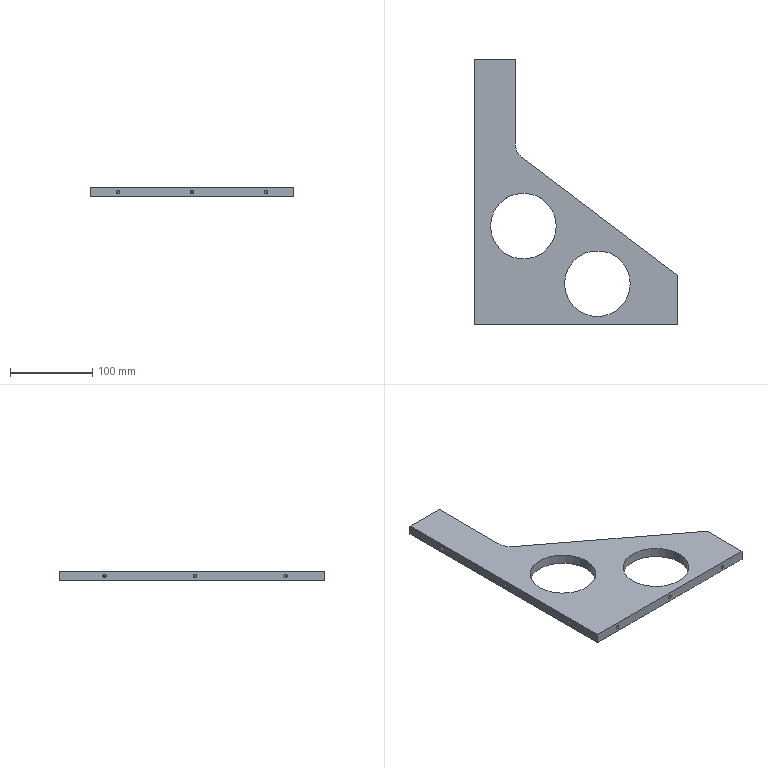Part | SolidWorks | features HoleWzd 2, ICE 2, Extrusion 1, Fillet 1 | 1 solid | 37 faces | box 248 x 323 x 12 mm | volume 393029 mm3 | cylinder 17 | cone 12 | plane 8 | commonest cylinder face diameters 4.2 x12 80 x4 40 x1
STEP:
#1=CARTESIAN_POINT('',(-111.6,238.,-2.1));
#2=VERTEX_POINT('',#1);
#3=CARTESIAN_POINT('',(-111.6,238.,2.1));
#4=VERTEX_POINT('',#3);
#5=CARTESIAN_POINT('',(-111.6,238.,0.));
#6=DIRECTION('',(-1.,0.,0.));
#7=DIRECTION('',(0.,0.,1.));
#8=AXIS2_PLACEMENT_3D('',#5,#6,#7);
#9=CIRCLE('',#8,2.1);
#10=EDGE_CURVE('',#2,#4,#9,.T.);
#11=ORIENTED_EDGE('',*,*,#10,.F.);
#12=CARTESIAN_POINT('',(-124.,238.,-2.1));
#13=VERTEX_POINT('',#12);
#14=CARTESIAN_POINT('',(-124.,238.,-2.1));
#15=DIRECTION('',(-1.,0.,0.));
#16=VECTOR('',#15,1000.);
#17=LINE('',#14,#16);
#18=EDGE_CURVE('',#2,#13,#17,.T.);
#19=ORIENTED_EDGE('',*,*,#18,.T.);
#20=CARTESIAN_POINT('',(-124.,238.,2.1));
#21=VERTEX_POINT('',#20);
#22=CARTESIAN_POINT('',(-124.,238.,0.));
#23=DIRECTION('',(-1.,0.,0.));
#24=DIRECTION('',(0.,0.,1.));
#25=AXIS2_PLACEMENT_3D('',#22,#23,#24);
#26=CIRCLE('',#25,2.1);
#27=EDGE_CURVE('',#13,#21,#26,.T.);
#28=ORIENTED_EDGE('',*,*,#27,.T.);
#29=CARTESIAN_POINT('',(-124.,238.,2.1));
#30=DIRECTION('',(-1.,0.,0.));
#31=VECTOR('',#30,1000.);
#32=LINE('',#29,#31);
#33=EDGE_CURVE('',#4,#21,#32,.T.);
#34=ORIENTED_EDGE('',*,*,#33,.F.);
#35=EDGE_LOOP('',(#11,#19,#28,#34));
#36=FACE_OUTER_BOUND('',#35,.T.);
#37=CARTESIAN_POINT('',(-124.,238.,0.));
#38=DIRECTION('',(-1.,0.,0.));
#39=DIRECTION('',(0.,0.,1.));
#40=AXIS2_PLACEMENT_3D('',#37,#38,#39);
#41=CYLINDRICAL_SURFACE('',#40,2.1);
#42=ADVANCED_FACE('',(#36),#41,.F.);
#43=CARTESIAN_POINT('',(-110.338,238.,0.));
#44=VERTEX_POINT('',#43);
#45=CARTESIAN_POINT('',(-111.6,238.,2.1));
#46=DIRECTION('',(-0.515,0.,0.8572));
#47=VECTOR('',#46,1000.);
#48=LINE('',#45,#47);
#49=EDGE_CURVE('',#44,#4,#48,.T.);
#50=ORIENTED_EDGE('',*,*,#49,.F.);
#51=CARTESIAN_POINT('',(-111.6,238.,-2.1));
#52=DIRECTION('',(-0.515,0.,-0.8572));
#53=VECTOR('',#52,1000.);
#54=LINE('',#51,#53);
#55=EDGE_CURVE('',#44,#2,#54,.T.);
#56=ORIENTED_EDGE('',*,*,#55,.T.);
#57=ORIENTED_EDGE('',*,*,#10,.T.);
#58=EDGE_LOOP('',(#50,#56,#57));
#59=FACE_OUTER_BOUND('',#58,.T.);
#60=CARTESIAN_POINT('',(-111.6,238.,0.));
#61=DIRECTION('',(-1.,0.,0.));
#62=DIRECTION('',(0.,0.,1.));
#63=AXIS2_PLACEMENT_3D('',#60,#61,#62);
#64=CONICAL_SURFACE('',#63,2.1,1.03);
#65=ADVANCED_FACE('',(#59),#64,.F.);
#66=CARTESIAN_POINT('',(-111.6,128.,-2.1));
#67=VERTEX_POINT('',#66);
#68=CARTESIAN_POINT('',(-111.6,128.,2.1));
#69=VERTEX_POINT('',#68);
#70=CARTESIAN_POINT('',(-111.6,128.,0.));
#71=DIRECTION('',(-1.,0.,0.));
#72=DIRECTION('',(0.,0.,1.));
#73=AXIS2_PLACEMENT_3D('',#70,#71,#72);
#74=CIRCLE('',#73,2.1);
#75=EDGE_CURVE('',#67,#69,#74,.T.);
#76=ORIENTED_EDGE('',*,*,#75,.F.);
#77=CARTESIAN_POINT('',(-124.,128.,-2.1));
#78=VERTEX_POINT('',#77);
#79=CARTESIAN_POINT('',(-124.,128.,-2.1));
#80=DIRECTION('',(-1.,0.,0.));
#81=VECTOR('',#80,1000.);
#82=LINE('',#79,#81);
#83=EDGE_CURVE('',#67,#78,#82,.T.);
#84=ORIENTED_EDGE('',*,*,#83,.T.);
#85=CARTESIAN_POINT('',(-124.,128.,2.1));
#86=VERTEX_POINT('',#85);
#87=CARTESIAN_POINT('',(-124.,128.,0.));
#88=DIRECTION('',(-1.,0.,0.));
#89=DIRECTION('',(0.,0.,1.));
#90=AXIS2_PLACEMENT_3D('',#87,#88,#89);
#91=CIRCLE('',#90,2.1);
#92=EDGE_CURVE('',#78,#86,#91,.T.);
#93=ORIENTED_EDGE('',*,*,#92,.T.);
#94=CARTESIAN_POINT('',(-124.,128.,2.1));
#95=DIRECTION('',(-1.,0.,0.));
#96=VECTOR('',#95,1000.);
#97=LINE('',#94,#96);
#98=EDGE_CURVE('',#69,#86,#97,.T.);
#99=ORIENTED_EDGE('',*,*,#98,.F.);
#100=EDGE_LOOP('',(#76,#84,#93,#99));
#101=FACE_OUTER_BOUND('',#100,.T.);
#102=CARTESIAN_POINT('',(-124.,128.,0.));
#103=DIRECTION('',(-1.,0.,0.));
#104=DIRECTION('',(0.,0.,1.));
#105=AXIS2_PLACEMENT_3D('',#102,#103,#104);
#106=CYLINDRICAL_SURFACE('',#105,2.1);
#107=ADVANCED_FACE('',(#101),#106,.F.);
#108=CARTESIAN_POINT('',(-110.338,128.,0.));
#109=VERTEX_POINT('',#108);
#110=CARTESIAN_POINT('',(-111.6,128.,2.1));
#111=DIRECTION('',(-0.515,0.,0.8572));
#112=VECTOR('',#111,1000.);
#113=LINE('',#110,#112);
#114=EDGE_CURVE('',#109,#69,#113,.T.);
#115=ORIENTED_EDGE('',*,*,#114,.F.);
#116=CARTESIAN_POINT('',(-111.6,128.,-2.1));
#117=DIRECTION('',(-0.515,0.,-0.8572));
#118=VECTOR('',#117,1000.);
#119=LINE('',#116,#118);
#120=EDGE_CURVE('',#109,#67,#119,.T.);
#121=ORIENTED_EDGE('',*,*,#120,.T.);
#122=ORIENTED_EDGE('',*,*,#75,.T.);
#123=EDGE_LOOP('',(#115,#121,#122));
#124=FACE_OUTER_BOUND('',#123,.T.);
#125=CARTESIAN_POINT('',(-111.6,128.,0.));
#126=DIRECTION('',(-1.,0.,0.));
#127=DIRECTION('',(0.,0.,1.));
#128=AXIS2_PLACEMENT_3D('',#125,#126,#127);
#129=CONICAL_SURFACE('',#128,2.1,1.03);
#130=ADVANCED_FACE('',(#124),#129,.F.);
#131=CARTESIAN_POINT('',(-111.6,18.,-2.1));
#132=VERTEX_POINT('',#131);
#133=CARTESIAN_POINT('',(-111.6,18.,2.1));
#134=VERTEX_POINT('',#133);
#135=CARTESIAN_POINT('',(-111.6,18.,0.));
#136=DIRECTION('',(-1.,0.,0.));
#137=DIRECTION('',(0.,0.,1.));
#138=AXIS2_PLACEMENT_3D('',#135,#136,#137);
#139=CIRCLE('',#138,2.1);
#140=EDGE_CURVE('',#132,#134,#139,.T.);
#141=ORIENTED_EDGE('',*,*,#140,.F.);
#142=CARTESIAN_POINT('',(-124.,18.,-2.1));
#143=VERTEX_POINT('',#142);
#144=CARTESIAN_POINT('',(-124.,18.,-2.1));
#145=DIRECTION('',(-1.,0.,0.));
#146=VECTOR('',#145,1000.);
#147=LINE('',#144,#146);
#148=EDGE_CURVE('',#132,#143,#147,.T.);
#149=ORIENTED_EDGE('',*,*,#148,.T.);
#150=CARTESIAN_POINT('',(-124.,18.,2.1));
#151=VERTEX_POINT('',#150);
#152=CARTESIAN_POINT('',(-124.,18.,0.));
#153=DIRECTION('',(-1.,0.,0.));
#154=DIRECTION('',(0.,0.,1.));
#155=AXIS2_PLACEMENT_3D('',#152,#153,#154);
#156=CIRCLE('',#155,2.1);
#157=EDGE_CURVE('',#143,#151,#156,.T.);
#158=ORIENTED_EDGE('',*,*,#157,.T.);
#159=CARTESIAN_POINT('',(-124.,18.,2.1));
#160=DIRECTION('',(-1.,0.,0.));
#161=VECTOR('',#160,1000.);
#162=LINE('',#159,#161);
#163=EDGE_CURVE('',#134,#151,#162,.T.);
#164=ORIENTED_EDGE('',*,*,#163,.F.);
#165=EDGE_LOOP('',(#141,#149,#158,#164));
#166=FACE_OUTER_BOUND('',#165,.T.);
#167=CARTESIAN_POINT('',(-124.,18.,0.));
#168=DIRECTION('',(-1.,0.,0.));
#169=DIRECTION('',(0.,0.,1.));
#170=AXIS2_PLACEMENT_3D('',#167,#168,#169);
#171=CYLINDRICAL_SURFACE('',#170,2.1);
#172=ADVANCED_FACE('',(#166),#171,.F.);
#173=CARTESIAN_POINT('',(-110.338,18.,0.));
#174=VERTEX_POINT('',#173);
#175=CARTESIAN_POINT('',(-111.6,18.,2.1));
#176=DIRECTION('',(-0.515,0.,0.8572));
#177=VECTOR('',#176,1000.);
#178=LINE('',#175,#177);
#179=EDGE_CURVE('',#174,#134,#178,.T.);
#180=ORIENTED_EDGE('',*,*,#179,.F.);
#181=CARTESIAN_POINT('',(-111.6,18.,-2.1));
#182=DIRECTION('',(-0.515,0.,-0.8572));
#183=VECTOR('',#182,1000.);
#184=LINE('',#181,#183);
#185=EDGE_CURVE('',#174,#132,#184,.T.);
#186=ORIENTED_EDGE('',*,*,#185,.T.);
#187=ORIENTED_EDGE('',*,*,#140,.T.);
#188=EDGE_LOOP('',(#180,#186,#187));
#189=FACE_OUTER_BOUND('',#188,.T.);
#190=CARTESIAN_POINT('',(-111.6,18.,0.));
#191=DIRECTION('',(-1.,0.,0.));
#192=DIRECTION('',(0.,0.,1.));
#193=AXIS2_PLACEMENT_3D('',#190,#191,#192);
#194=CONICAL_SURFACE('',#193,2.1,1.03);
#195=ADVANCED_FACE('',(#189),#194,.F.);
#196=CARTESIAN_POINT('',(90.,-17.6,2.1));
#197=VERTEX_POINT('',#196);
#198=CARTESIAN_POINT('',(90.,-17.6,-2.1));
#199=VERTEX_POINT('',#198);
#200=CARTESIAN_POINT('',(90.,-17.6,0.));
#201=DIRECTION('',(0.,-1.,0.));
#202=DIRECTION('',(0.,0.,-1.));
#203=AXIS2_PLACEMENT_3D('',#200,#201,#202);
#204=CIRCLE('',#203,2.1);
#205=EDGE_CURVE('',#197,#199,#204,.T.);
#206=ORIENTED_EDGE('',*,*,#205,.F.);
#207=CARTESIAN_POINT('',(90.,-30.,2.1));
#208=VERTEX_POINT('',#207);
#209=CARTESIAN_POINT('',(90.,-30.,2.1));
#210=DIRECTION('',(0.,-1.,0.));
#211=VECTOR('',#210,1000.);
#212=LINE('',#209,#211);
#213=EDGE_CURVE('',#197,#208,#212,.T.);
#214=ORIENTED_EDGE('',*,*,#213,.T.);
#215=CARTESIAN_POINT('',(90.,-30.,-2.1));
#216=VERTEX_POINT('',#215);
#217=CARTESIAN_POINT('',(90.,-30.,0.));
#218=DIRECTION('',(0.,-1.,0.));
#219=DIRECTION('',(0.,0.,-1.));
#220=AXIS2_PLACEMENT_3D('',#217,#218,#219);
#221=CIRCLE('',#220,2.1);
#222=EDGE_CURVE('',#208,#216,#221,.T.);
#223=ORIENTED_EDGE('',*,*,#222,.T.);
#224=CARTESIAN_POINT('',(90.,-30.,-2.1));
#225=DIRECTION('',(0.,-1.,0.));
#226=VECTOR('',#225,1000.);
#227=LINE('',#224,#226);
#228=EDGE_CURVE('',#199,#216,#227,.T.);
#229=ORIENTED_EDGE('',*,*,#228,.F.);
#230=EDGE_LOOP('',(#206,#214,#223,#229));
#231=FACE_OUTER_BOUND('',#230,.T.);
#232=CARTESIAN_POINT('',(90.,-30.,0.));
#233=DIRECTION('',(0.,-1.,0.));
#234=DIRECTION('',(0.,0.,-1.));
#235=AXIS2_PLACEMENT_3D('',#232,#233,#234);
#236=CYLINDRICAL_SURFACE('',#235,2.1);
#237=ADVANCED_FACE('',(#231),#236,.F.);
#238=CARTESIAN_POINT('',(90.,-16.338,0.));
#239=VERTEX_POINT('',#238);
#240=CARTESIAN_POINT('',(90.,-17.6,-2.1));
#241=DIRECTION('',(0.,-0.515,-0.8572));
#242=VECTOR('',#241,1000.);
#243=LINE('',#240,#242);
#244=EDGE_CURVE('',#239,#199,#243,.T.);
#245=ORIENTED_EDGE('',*,*,#244,.F.);
#246=CARTESIAN_POINT('',(90.,-17.6,2.1));
#247=DIRECTION('',(0.,-0.515,0.8572));
#248=VECTOR('',#247,1000.);
#249=LINE('',#246,#248);
#250=EDGE_CURVE('',#239,#197,#249,.T.);
#251=ORIENTED_EDGE('',*,*,#250,.T.);
#252=ORIENTED_EDGE('',*,*,#205,.T.);
#253=EDGE_LOOP('',(#245,#251,#252));
#254=FACE_OUTER_BOUND('',#253,.T.);
#255=CARTESIAN_POINT('',(90.,-17.6,0.));
#256=DIRECTION('',(0.,-1.,0.));
#257=DIRECTION('',(0.,0.,-1.));
#258=AXIS2_PLACEMENT_3D('',#255,#256,#257);
#259=CONICAL_SURFACE('',#258,2.1,1.03);
#260=ADVANCED_FACE('',(#254),#259,.F.);
#261=CARTESIAN_POINT('',(0.,-17.6,2.1));
#262=VERTEX_POINT('',#261);
#263=CARTESIAN_POINT('',(0.,-17.6,-2.1));
#264=VERTEX_POINT('',#263);
#265=CARTESIAN_POINT('',(0.,-17.6,0.));
#266=DIRECTION('',(0.,-1.,0.));
#267=DIRECTION('',(0.,0.,-1.));
#268=AXIS2_PLACEMENT_3D('',#265,#266,#267);
#269=CIRCLE('',#268,2.1);
#270=EDGE_CURVE('',#262,#264,#269,.T.);
#271=ORIENTED_EDGE('',*,*,#270,.F.);
#272=CARTESIAN_POINT('',(0.,-30.,2.1));
#273=VERTEX_POINT('',#272);
#274=CARTESIAN_POINT('',(0.,-30.,2.1));
#275=DIRECTION('',(0.,-1.,0.));
#276=VECTOR('',#275,1000.);
#277=LINE('',#274,#276);
#278=EDGE_CURVE('',#262,#273,#277,.T.);
#279=ORIENTED_EDGE('',*,*,#278,.T.);
#280=CARTESIAN_POINT('',(0.,-30.,-2.1));
#281=VERTEX_POINT('',#280);
#282=CARTESIAN_POINT('',(0.,-30.,0.));
#283=DIRECTION('',(0.,-1.,0.));
#284=DIRECTION('',(0.,0.,-1.));
#285=AXIS2_PLACEMENT_3D('',#282,#283,#284);
#286=CIRCLE('',#285,2.1);
#287=EDGE_CURVE('',#273,#281,#286,.T.);
#288=ORIENTED_EDGE('',*,*,#287,.T.);
#289=CARTESIAN_POINT('',(0.,-30.,-2.1));
#290=DIRECTION('',(0.,-1.,0.));
#291=VECTOR('',#290,1000.);
#292=LINE('',#289,#291);
#293=EDGE_CURVE('',#264,#281,#292,.T.);
#294=ORIENTED_EDGE('',*,*,#293,.F.);
#295=EDGE_LOOP('',(#271,#279,#288,#294));
#296=FACE_OUTER_BOUND('',#295,.T.);
#297=CARTESIAN_POINT('',(0.,-30.,0.));
#298=DIRECTION('',(0.,-1.,0.));
#299=DIRECTION('',(0.,0.,-1.));
#300=AXIS2_PLACEMENT_3D('',#297,#298,#299);
#301=CYLINDRICAL_SURFACE('',#300,2.1);
#302=ADVANCED_FACE('',(#296),#301,.F.);
#303=CARTESIAN_POINT('',(0.,-16.338,0.));
#304=VERTEX_POINT('',#303);
#305=CARTESIAN_POINT('',(0.,-17.6,-2.1));
#306=DIRECTION('',(0.,-0.515,-0.8572));
#307=VECTOR('',#306,1000.);
#308=LINE('',#305,#307);
#309=EDGE_CURVE('',#304,#264,#308,.T.);
#310=ORIENTED_EDGE('',*,*,#309,.F.);
#311=CARTESIAN_POINT('',(0.,-17.6,2.1));
#312=DIRECTION('',(0.,-0.515,0.8572));
#313=VECTOR('',#312,1000.);
#314=LINE('',#311,#313);
#315=EDGE_CURVE('',#304,#262,#314,.T.);
#316=ORIENTED_EDGE('',*,*,#315,.T.);
#317=ORIENTED_EDGE('',*,*,#270,.T.);
#318=EDGE_LOOP('',(#310,#316,#317));
#319=FACE_OUTER_BOUND('',#318,.T.);
#320=CARTESIAN_POINT('',(0.,-17.6,0.));
#321=DIRECTION('',(0.,-1.,0.));
#322=DIRECTION('',(0.,0.,-1.));
#323=AXIS2_PLACEMENT_3D('',#320,#321,#322);
#324=CONICAL_SURFACE('',#323,2.1,1.03);
#325=ADVANCED_FACE('',(#319),#324,.F.);
#326=CARTESIAN_POINT('',(-90.,-17.6,2.1));
#327=VERTEX_POINT('',#326);
#328=CARTESIAN_POINT('',(-90.,-17.6,-2.1));
#329=VERTEX_POINT('',#328);
#330=CARTESIAN_POINT('',(-90.,-17.6,0.));
#331=DIRECTION('',(0.,-1.,0.));
#332=DIRECTION('',(0.,0.,-1.));
#333=AXIS2_PLACEMENT_3D('',#330,#331,#332);
#334=CIRCLE('',#333,2.1);
#335=EDGE_CURVE('',#327,#329,#334,.T.);
#336=ORIENTED_EDGE('',*,*,#335,.F.);
#337=CARTESIAN_POINT('',(-90.,-30.,2.1));
#338=VERTEX_POINT('',#337);
#339=CARTESIAN_POINT('',(-90.,-30.,2.1));
#340=DIRECTION('',(0.,-1.,0.));
#341=VECTOR('',#340,1000.);
#342=LINE('',#339,#341);
#343=EDGE_CURVE('',#327,#338,#342,.T.);
#344=ORIENTED_EDGE('',*,*,#343,.T.);
#345=CARTESIAN_POINT('',(-90.,-30.,-2.1));
#346=VERTEX_POINT('',#345);
#347=CARTESIAN_POINT('',(-90.,-30.,0.));
#348=DIRECTION('',(0.,-1.,0.));
#349=DIRECTION('',(0.,0.,-1.));
#350=AXIS2_PLACEMENT_3D('',#347,#348,#349);
#351=CIRCLE('',#350,2.1);
#352=EDGE_CURVE('',#338,#346,#351,.T.);
#353=ORIENTED_EDGE('',*,*,#352,.T.);
#354=CARTESIAN_POINT('',(-90.,-30.,-2.1));
#355=DIRECTION('',(0.,-1.,0.));
#356=VECTOR('',#355,1000.);
#357=LINE('',#354,#356);
#358=EDGE_CURVE('',#329,#346,#357,.T.);
#359=ORIENTED_EDGE('',*,*,#358,.F.);
#360=EDGE_LOOP('',(#336,#344,#353,#359));
#361=FACE_OUTER_BOUND('',#360,.T.);
#362=CARTESIAN_POINT('',(-90.,-30.,0.));
#363=DIRECTION('',(0.,-1.,0.));
#364=DIRECTION('',(0.,0.,-1.));
#365=AXIS2_PLACEMENT_3D('',#362,#363,#364);
#366=CYLINDRICAL_SURFACE('',#365,2.1);
#367=ADVANCED_FACE('',(#361),#366,.F.);
#368=CARTESIAN_POINT('',(-90.,-16.338,0.));
#369=VERTEX_POINT('',#368);
#370=CARTESIAN_POINT('',(-90.,-17.6,-2.1));
#371=DIRECTION('',(0.,-0.515,-0.8572));
#372=VECTOR('',#371,1000.);
#373=LINE('',#370,#372);
#374=EDGE_CURVE('',#369,#329,#373,.T.);
#375=ORIENTED_EDGE('',*,*,#374,.F.);
#376=CARTESIAN_POINT('',(-90.,-17.6,2.1));
#377=DIRECTION('',(0.,-0.515,0.8572));
#378=VECTOR('',#377,1000.);
#379=LINE('',#376,#378);
#380=EDGE_CURVE('',#369,#327,#379,.T.);
#381=ORIENTED_EDGE('',*,*,#380,.T.);
#382=ORIENTED_EDGE('',*,*,#335,.T.);
#383=EDGE_LOOP('',(#375,#381,#382));
#384=FACE_OUTER_BOUND('',#383,.T.);
#385=CARTESIAN_POINT('',(-90.,-17.6,0.));
#386=DIRECTION('',(0.,-1.,0.));
#387=DIRECTION('',(0.,0.,-1.));
#388=AXIS2_PLACEMENT_3D('',#385,#386,#387);
#389=CONICAL_SURFACE('',#388,2.1,1.03);
#390=ADVANCED_FACE('',(#384),#389,.F.);
#391=CARTESIAN_POINT('',(66.,20.,6.));
#392=VERTEX_POINT('',#391);
#393=CARTESIAN_POINT('',(-14.,20.,6.));
#394=VERTEX_POINT('',#393);
#395=CARTESIAN_POINT('',(26.,20.,6.));
#396=DIRECTION('',(0.,0.,-1.));
#397=DIRECTION('',(-1.,0.,0.));
#398=AXIS2_PLACEMENT_3D('',#395,#396,#397);
#399=CIRCLE('',#398,40.);
#400=EDGE_CURVE('',#392,#394,#399,.T.);
#401=ORIENTED_EDGE('',*,*,#400,.F.);
#402=CARTESIAN_POINT('',(66.,20.,-6.));
#403=VERTEX_POINT('',#402);
#404=CARTESIAN_POINT('',(66.,20.,6.));
#405=DIRECTION('',(0.,0.,-1.));
#406=VECTOR('',#405,1000.);
#407=LINE('',#404,#406);
#408=EDGE_CURVE('',#392,#403,#407,.T.);
#409=ORIENTED_EDGE('',*,*,#408,.T.);
#410=CARTESIAN_POINT('',(-14.,20.,-6.));
#411=VERTEX_POINT('',#410);
#412=CARTESIAN_POINT('',(26.,20.,-6.));
#413=DIRECTION('',(0.,0.,-1.));
#414=DIRECTION('',(-1.,0.,0.));
#415=AXIS2_PLACEMENT_3D('',#412,#413,#414);
#416=CIRCLE('',#415,40.);
#417=EDGE_CURVE('',#403,#411,#416,.T.);
#418=ORIENTED_EDGE('',*,*,#417,.T.);
#419=CARTESIAN_POINT('',(-14.,20.,6.));
#420=DIRECTION('',(0.,0.,-1.));
#421=VECTOR('',#420,1000.);
#422=LINE('',#419,#421);
#423=EDGE_CURVE('',#394,#411,#422,.T.);
#424=ORIENTED_EDGE('',*,*,#423,.F.);
#425=EDGE_LOOP('',(#401,#409,#418,#424));
#426=FACE_OUTER_BOUND('',#425,.T.);
#427=CARTESIAN_POINT('',(26.,20.,6.));
#428=DIRECTION('',(0.,0.,-1.));
#429=DIRECTION('',(-1.,0.,0.));
#430=AXIS2_PLACEMENT_3D('',#427,#428,#429);
#431=CYLINDRICAL_SURFACE('',#430,40.);
#432=ADVANCED_FACE('',(#426),#431,.F.);
#433=CARTESIAN_POINT('',(-24.,90.,6.));
#434=VERTEX_POINT('',#433);
#435=CARTESIAN_POINT('',(-104.,90.,6.));
#436=VERTEX_POINT('',#435);
#437=CARTESIAN_POINT('',(-64.,90.,6.));
#438=DIRECTION('',(0.,0.,-1.));
#439=DIRECTION('',(-1.,0.,0.));
#440=AXIS2_PLACEMENT_3D('',#437,#438,#439);
#441=CIRCLE('',#440,40.);
#442=EDGE_CURVE('',#434,#436,#441,.T.);
#443=ORIENTED_EDGE('',*,*,#442,.F.);
#444=CARTESIAN_POINT('',(-24.,90.,-6.));
#445=VERTEX_POINT('',#444);
#446=CARTESIAN_POINT('',(-24.,90.,6.));
#447=DIRECTION('',(0.,0.,-1.));
#448=VECTOR('',#447,1000.);
#449=LINE('',#446,#448);
#450=EDGE_CURVE('',#434,#445,#449,.T.);
#451=ORIENTED_EDGE('',*,*,#450,.T.);
#452=CARTESIAN_POINT('',(-104.,90.,-6.));
#453=VERTEX_POINT('',#452);
#454=CARTESIAN_POINT('',(-64.,90.,-6.));
#455=DIRECTION('',(0.,0.,-1.));
#456=DIRECTION('',(-1.,0.,0.));
#457=AXIS2_PLACEMENT_3D('',#454,#455,#456);
#458=CIRCLE('',#457,40.);
#459=EDGE_CURVE('',#445,#453,#458,.T.);
#460=ORIENTED_EDGE('',*,*,#459,.T.);
#461=CARTESIAN_POINT('',(-104.,90.,6.));
#462=DIRECTION('',(0.,0.,-1.));
#463=VECTOR('',#462,1000.);
#464=LINE('',#461,#463);
#465=EDGE_CURVE('',#436,#453,#464,.T.);
#466=ORIENTED_EDGE('',*,*,#465,.F.);
#467=EDGE_LOOP('',(#443,#451,#460,#466));
#468=FACE_OUTER_BOUND('',#467,.T.);
#469=CARTESIAN_POINT('',(-64.,90.,6.));
#470=DIRECTION('',(0.,0.,-1.));
#471=DIRECTION('',(-1.,0.,0.));
#472=AXIS2_PLACEMENT_3D('',#469,#470,#471);
#473=CYLINDRICAL_SURFACE('',#472,40.);
#474=ADVANCED_FACE('',(#468),#473,.F.);
#475=CARTESIAN_POINT('',(124.,-30.,-6.));
#476=VERTEX_POINT('',#475);
#477=CARTESIAN_POINT('',(124.,30.,-6.));
#478=VERTEX_POINT('',#477);
#479=CARTESIAN_POINT('',(124.,-30.,-6.));
#480=DIRECTION('',(0.,1.,0.));
#481=VECTOR('',#480,1000.);
#482=LINE('',#479,#481);
#483=EDGE_CURVE('',#476,#478,#482,.T.);
#484=ORIENTED_EDGE('',*,*,#483,.T.);
#485=CARTESIAN_POINT('',(124.,30.,6.));
#486=VERTEX_POINT('',#485);
#487=CARTESIAN_POINT('',(124.,30.,6.));
#488=DIRECTION('',(0.,0.,-1.));
#489=VECTOR('',#488,1000.);
#490=LINE('',#487,#489);
#491=EDGE_CURVE('',#486,#478,#490,.T.);
#492=ORIENTED_EDGE('',*,*,#491,.F.);
#493=CARTESIAN_POINT('',(124.,-30.,6.));
#494=VERTEX_POINT('',#493);
#495=CARTESIAN_POINT('',(124.,-30.,6.));
#496=DIRECTION('',(0.,1.,0.));
#497=VECTOR('',#496,1000.);
#498=LINE('',#495,#497);
#499=EDGE_CURVE('',#494,#486,#498,.T.);
#500=ORIENTED_EDGE('',*,*,#499,.F.);
#501=CARTESIAN_POINT('',(124.,-30.,6.));
#502=DIRECTION('',(0.,0.,-1.));
#503=VECTOR('',#502,1000.);
#504=LINE('',#501,#503);
#505=EDGE_CURVE('',#494,#476,#504,.T.);
#506=ORIENTED_EDGE('',*,*,#505,.T.);
#507=EDGE_LOOP('',(#484,#492,#500,#506));
#508=FACE_OUTER_BOUND('',#507,.T.);
#509=CARTESIAN_POINT('',(124.,-30.,6.));
#510=DIRECTION('',(-1.,0.,0.));
#511=DIRECTION('',(0.,0.,1.));
#512=AXIS2_PLACEMENT_3D('',#509,#510,#511);
#513=PLANE('',#512);
#514=ADVANCED_FACE('',(#508),#513,.F.);
#515=CARTESIAN_POINT('',(-124.,238.,0.));
#516=DIRECTION('',(-1.,0.,0.));
#517=DIRECTION('',(0.,0.,1.));
#518=AXIS2_PLACEMENT_3D('',#515,#516,#517);
#519=CIRCLE('',#518,2.1);
#520=EDGE_CURVE('',#21,#13,#519,.T.);
#521=ORIENTED_EDGE('',*,*,#520,.F.);
#522=ORIENTED_EDGE('',*,*,#27,.F.);
#523=EDGE_LOOP('',(#521,#522));
#524=FACE_BOUND('',#523,.T.);
#525=CARTESIAN_POINT('',(-124.,128.,0.));
#526=DIRECTION('',(-1.,0.,0.));
#527=DIRECTION('',(0.,0.,1.));
#528=AXIS2_PLACEMENT_3D('',#525,#526,#527);
#529=CIRCLE('',#528,2.1);
#530=EDGE_CURVE('',#86,#78,#529,.T.);
#531=ORIENTED_EDGE('',*,*,#530,.F.);
#532=ORIENTED_EDGE('',*,*,#92,.F.);
#533=EDGE_LOOP('',(#531,#532));
#534=FACE_BOUND('',#533,.T.);
#535=CARTESIAN_POINT('',(-124.,18.,0.));
#536=DIRECTION('',(-1.,0.,0.));
#537=DIRECTION('',(0.,0.,1.));
#538=AXIS2_PLACEMENT_3D('',#535,#536,#537);
#539=CIRCLE('',#538,2.1);
#540=EDGE_CURVE('',#151,#143,#539,.T.);
#541=ORIENTED_EDGE('',*,*,#540,.F.);
#542=ORIENTED_EDGE('',*,*,#157,.F.);
#543=EDGE_LOOP('',(#541,#542));
#544=FACE_BOUND('',#543,.T.);
#545=CARTESIAN_POINT('',(-124.,293.,-6.));
#546=VERTEX_POINT('',#545);
#547=CARTESIAN_POINT('',(-124.,-30.,-6.));
#548=VERTEX_POINT('',#547);
#549=CARTESIAN_POINT('',(-124.,-30.,-6.));
#550=DIRECTION('',(0.,-1.,0.));
#551=VECTOR('',#550,1000.);
#552=LINE('',#549,#551);
#553=EDGE_CURVE('',#546,#548,#552,.T.);
#554=ORIENTED_EDGE('',*,*,#553,.T.);
#555=CARTESIAN_POINT('',(-124.,-30.,6.));
#556=VERTEX_POINT('',#555);
#557=CARTESIAN_POINT('',(-124.,-30.,6.));
#558=DIRECTION('',(0.,0.,-1.));
#559=VECTOR('',#558,1000.);
#560=LINE('',#557,#559);
#561=EDGE_CURVE('',#556,#548,#560,.T.);
#562=ORIENTED_EDGE('',*,*,#561,.F.);
#563=CARTESIAN_POINT('',(-124.,293.,6.));
#564=VERTEX_POINT('',#563);
#565=CARTESIAN_POINT('',(-124.,-30.,6.));
#566=DIRECTION('',(0.,-1.,0.));
#567=VECTOR('',#566,1000.);
#568=LINE('',#565,#567);
#569=EDGE_CURVE('',#564,#556,#568,.T.);
#570=ORIENTED_EDGE('',*,*,#569,.F.);
#571=CARTESIAN_POINT('',(-124.,293.,367.487));
#572=DIRECTION('',(0.,0.,-1.));
#573=VECTOR('',#572,1000.);
#574=LINE('',#571,#573);
#575=EDGE_CURVE('',#564,#546,#574,.T.);
#576=ORIENTED_EDGE('',*,*,#575,.T.);
#577=EDGE_LOOP('',(#554,#562,#570,#576));
#578=FACE_OUTER_BOUND('',#577,.T.);
#579=CARTESIAN_POINT('',(-124.,-30.,6.));
#580=DIRECTION('',(1.,0.,0.));
#581=DIRECTION('',(0.,0.,-1.));
#582=AXIS2_PLACEMENT_3D('',#579,#580,#581);
#583=PLANE('',#582);
#584=ADVANCED_FACE('',(#524,#534,#544,#578),#583,.F.);
#585=CARTESIAN_POINT('',(90.,-30.,0.));
#586=DIRECTION('',(0.,-1.,0.));
#587=DIRECTION('',(0.,0.,-1.));
#588=AXIS2_PLACEMENT_3D('',#585,#586,#587);
#589=CIRCLE('',#588,2.1);
#590=EDGE_CURVE('',#216,#208,#589,.T.);
#591=ORIENTED_EDGE('',*,*,#590,.F.);
#592=ORIENTED_EDGE('',*,*,#222,.F.);
#593=EDGE_LOOP('',(#591,#592));
#594=FACE_BOUND('',#593,.T.);
#595=CARTESIAN_POINT('',(0.,-30.,0.));
#596=DIRECTION('',(0.,-1.,0.));
#597=DIRECTION('',(0.,0.,-1.));
#598=AXIS2_PLACEMENT_3D('',#595,#596,#597);
#599=CIRCLE('',#598,2.1);
#600=EDGE_CURVE('',#281,#273,#599,.T.);
#601=ORIENTED_EDGE('',*,*,#600,.F.);
#602=ORIENTED_EDGE('',*,*,#287,.F.);
#603=EDGE_LOOP('',(#601,#602));
#604=FACE_BOUND('',#603,.T.);
#605=CARTESIAN_POINT('',(-90.,-30.,0.));
#606=DIRECTION('',(0.,-1.,0.));
#607=DIRECTION('',(0.,0.,-1.));
#608=AXIS2_PLACEMENT_3D('',#605,#606,#607);
#609=CIRCLE('',#608,2.1);
#610=EDGE_CURVE('',#346,#338,#609,.T.);
#611=ORIENTED_EDGE('',*,*,#610,.F.);
#612=ORIENTED_EDGE('',*,*,#352,.F.);
#613=EDGE_LOOP('',(#611,#612));
#614=FACE_BOUND('',#613,.T.);
#615=CARTESIAN_POINT('',(-124.,-30.,-6.));
#616=DIRECTION('',(1.,0.,0.));
#617=VECTOR('',#616,1000.);
#618=LINE('',#615,#617);
#619=EDGE_CURVE('',#548,#476,#618,.T.);
#620=ORIENTED_EDGE('',*,*,#619,.T.);
#621=ORIENTED_EDGE('',*,*,#505,.F.);
#622=CARTESIAN_POINT('',(-124.,-30.,6.));
#623=DIRECTION('',(1.,0.,0.));
#624=VECTOR('',#623,1000.);
#625=LINE('',#622,#624);
#626=EDGE_CURVE('',#556,#494,#625,.T.);
#627=ORIENTED_EDGE('',*,*,#626,.F.);
#628=ORIENTED_EDGE('',*,*,#561,.T.);
#629=EDGE_LOOP('',(#620,#621,#627,#628));
#630=FACE_OUTER_BOUND('',#629,.T.);
#631=CARTESIAN_POINT('',(-124.,-30.,6.));
#632=DIRECTION('',(0.,1.,0.));
#633=DIRECTION('',(0.,0.,1.));
#634=AXIS2_PLACEMENT_3D('',#631,#632,#633);
#635=PLANE('',#634);
#636=ADVANCED_FACE('',(#594,#604,#614,#630),#635,.F.);
#637=CARTESIAN_POINT('',(26.,20.,6.));
#638=DIRECTION('',(0.,0.,-1.));
#639=DIRECTION('',(-1.,0.,0.));
#640=AXIS2_PLACEMENT_3D('',#637,#638,#639);
#641=CIRCLE('',#640,40.);
#642=EDGE_CURVE('',#394,#392,#641,.T.);
#643=ORIENTED_EDGE('',*,*,#642,.T.);
#644=ORIENTED_EDGE('',*,*,#400,.T.);
#645=EDGE_LOOP('',(#643,#644));
#646=FACE_BOUND('',#645,.T.);
#647=CARTESIAN_POINT('',(-64.,90.,6.));
#648=DIRECTION('',(0.,0.,-1.));
#649=DIRECTION('',(-1.,0.,0.));
#650=AXIS2_PLACEMENT_3D('',#647,#648,#649);
#651=CIRCLE('',#650,40.);
#652=EDGE_CURVE('',#436,#434,#651,.T.);
#653=ORIENTED_EDGE('',*,*,#652,.T.);
#654=ORIENTED_EDGE('',*,*,#442,.T.);
#655=EDGE_LOOP('',(#653,#654));
#656=FACE_BOUND('',#655,.T.);
#657=ORIENTED_EDGE('',*,*,#499,.T.);
#658=CARTESIAN_POINT('',(-66.077,173.998,6.));
#659=VERTEX_POINT('',#658);
#660=CARTESIAN_POINT('',(124.,30.,6.));
#661=DIRECTION('',(-0.7971,0.6039,0.));
#662=VECTOR('',#661,1000.);
#663=LINE('',#660,#662);
#664=EDGE_CURVE('',#486,#659,#663,.T.);
#665=ORIENTED_EDGE('',*,*,#664,.T.);
#666=CARTESIAN_POINT('',(-74.,189.94,6.));
#667=VERTEX_POINT('',#666);
#668=CARTESIAN_POINT('',(-54.,189.94,6.));
#669=DIRECTION('',(0.,0.,-1.));
#670=DIRECTION('',(-1.,0.,0.));
#671=AXIS2_PLACEMENT_3D('',#668,#669,#670);
#672=CIRCLE('',#671,20.);
#673=EDGE_CURVE('',#659,#667,#672,.T.);
#674=ORIENTED_EDGE('',*,*,#673,.T.);
#675=CARTESIAN_POINT('',(-74.,293.,6.));
#676=VERTEX_POINT('',#675);
#677=CARTESIAN_POINT('',(-74.,180.,6.));
#678=DIRECTION('',(0.,1.,0.));
#679=VECTOR('',#678,1000.);
#680=LINE('',#677,#679);
#681=EDGE_CURVE('',#667,#676,#680,.T.);
#682=ORIENTED_EDGE('',*,*,#681,.T.);
#683=CARTESIAN_POINT('',(-74.,293.,6.));
#684=DIRECTION('',(-1.,0.,0.));
#685=VECTOR('',#684,1000.);
#686=LINE('',#683,#685);
#687=EDGE_CURVE('',#676,#564,#686,.T.);
#688=ORIENTED_EDGE('',*,*,#687,.T.);
#689=ORIENTED_EDGE('',*,*,#569,.T.);
#690=ORIENTED_EDGE('',*,*,#626,.T.);
#691=EDGE_LOOP('',(#657,#665,#674,#682,#688,#689,#690));
#692=FACE_OUTER_BOUND('',#691,.T.);
#693=CARTESIAN_POINT('',(0.,0.,6.));
#694=DIRECTION('',(0.,0.,-1.));
#695=DIRECTION('',(-1.,0.,0.));
#696=AXIS2_PLACEMENT_3D('',#693,#694,#695);
#697=PLANE('',#696);
#698=ADVANCED_FACE('',(#646,#656,#692),#697,.F.);
#699=CARTESIAN_POINT('',(26.,20.,-6.));
#700=DIRECTION('',(0.,0.,-1.));
#701=DIRECTION('',(-1.,0.,0.));
#702=AXIS2_PLACEMENT_3D('',#699,#700,#701);
#703=CIRCLE('',#702,40.);
#704=EDGE_CURVE('',#411,#403,#703,.T.);
#705=ORIENTED_EDGE('',*,*,#704,.F.);
#706=ORIENTED_EDGE('',*,*,#417,.F.);
#707=EDGE_LOOP('',(#705,#706));
#708=FACE_BOUND('',#707,.T.);
#709=CARTESIAN_POINT('',(-64.,90.,-6.));
#710=DIRECTION('',(0.,0.,-1.));
#711=DIRECTION('',(-1.,0.,0.));
#712=AXIS2_PLACEMENT_3D('',#709,#710,#711);
#713=CIRCLE('',#712,40.);
#714=EDGE_CURVE('',#453,#445,#713,.T.);
#715=ORIENTED_EDGE('',*,*,#714,.F.);
#716=ORIENTED_EDGE('',*,*,#459,.F.);
#717=EDGE_LOOP('',(#715,#716));
#718=FACE_BOUND('',#717,.T.);
#719=ORIENTED_EDGE('',*,*,#483,.F.);
#720=ORIENTED_EDGE('',*,*,#619,.F.);
#721=ORIENTED_EDGE('',*,*,#553,.F.);
#722=CARTESIAN_POINT('',(-74.,293.,-6.));
#723=VERTEX_POINT('',#722);
#724=CARTESIAN_POINT('',(-74.,293.,-6.));
#725=DIRECTION('',(1.,0.,0.));
#726=VECTOR('',#725,1000.);
#727=LINE('',#724,#726);
#728=EDGE_CURVE('',#546,#723,#727,.T.);
#729=ORIENTED_EDGE('',*,*,#728,.T.);
#730=CARTESIAN_POINT('',(-74.,189.94,-6.));
#731=VERTEX_POINT('',#730);
#732=CARTESIAN_POINT('',(-74.,180.,-6.));
#733=DIRECTION('',(0.,-1.,0.));
#734=VECTOR('',#733,1000.);
#735=LINE('',#732,#734);
#736=EDGE_CURVE('',#723,#731,#735,.T.);
#737=ORIENTED_EDGE('',*,*,#736,.T.);
#738=CARTESIAN_POINT('',(-66.077,173.998,-6.));
#739=VERTEX_POINT('',#738);
#740=CARTESIAN_POINT('',(-54.,189.94,-6.));
#741=DIRECTION('',(0.,0.,1.));
#742=DIRECTION('',(-1.,0.,0.));
#743=AXIS2_PLACEMENT_3D('',#740,#741,#742);
#744=CIRCLE('',#743,20.);
#745=EDGE_CURVE('',#731,#739,#744,.T.);
#746=ORIENTED_EDGE('',*,*,#745,.T.);
#747=CARTESIAN_POINT('',(124.,30.,-6.));
#748=DIRECTION('',(0.7971,-0.6039,0.));
#749=VECTOR('',#748,1000.);
#750=LINE('',#747,#749);
#751=EDGE_CURVE('',#739,#478,#750,.T.);
#752=ORIENTED_EDGE('',*,*,#751,.T.);
#753=EDGE_LOOP('',(#719,#720,#721,#729,#737,#746,#752));
#754=FACE_OUTER_BOUND('',#753,.T.);
#755=CARTESIAN_POINT('',(0.,0.,-6.));
#756=DIRECTION('',(0.,0.,-1.));
#757=DIRECTION('',(-1.,0.,0.));
#758=AXIS2_PLACEMENT_3D('',#755,#756,#757);
#759=PLANE('',#758);
#760=ADVANCED_FACE('',(#708,#718,#754),#759,.T.);
#761=ORIENTED_EDGE('',*,*,#751,.F.);
#762=CARTESIAN_POINT('',(-66.077,173.998,6.));
#763=DIRECTION('',(0.,0.,1.));
#764=VECTOR('',#763,1000.);
#765=LINE('',#762,#764);
#766=EDGE_CURVE('',#739,#659,#765,.T.);
#767=ORIENTED_EDGE('',*,*,#766,.T.);
#768=ORIENTED_EDGE('',*,*,#664,.F.);
#769=ORIENTED_EDGE('',*,*,#491,.T.);
#770=EDGE_LOOP('',(#761,#767,#768,#769));
#771=FACE_OUTER_BOUND('',#770,.T.);
#772=CARTESIAN_POINT('',(124.,30.,367.487));
#773=DIRECTION('',(0.6039,0.7971,0.));
#774=DIRECTION('',(-0.7971,0.6039,0.));
#775=AXIS2_PLACEMENT_3D('',#772,#773,#774);
#776=PLANE('',#775);
#777=ADVANCED_FACE('',(#771),#776,.T.);
#778=ORIENTED_EDGE('',*,*,#681,.F.);
#779=CARTESIAN_POINT('',(-74.,189.94,-6.));
#780=DIRECTION('',(0.,0.,-1.));
#781=VECTOR('',#780,1000.);
#782=LINE('',#779,#781);
#783=EDGE_CURVE('',#667,#731,#782,.T.);
#784=ORIENTED_EDGE('',*,*,#783,.T.);
#785=ORIENTED_EDGE('',*,*,#736,.F.);
#786=CARTESIAN_POINT('',(-74.,293.,367.487));
#787=DIRECTION('',(0.,0.,-1.));
#788=VECTOR('',#787,1000.);
#789=LINE('',#786,#788);
#790=EDGE_CURVE('',#676,#723,#789,.T.);
#791=ORIENTED_EDGE('',*,*,#790,.F.);
#792=EDGE_LOOP('',(#778,#784,#785,#791));
#793=FACE_OUTER_BOUND('',#792,.T.);
#794=CARTESIAN_POINT('',(-74.,180.,367.487));
#795=DIRECTION('',(1.,0.,0.));
#796=DIRECTION('',(0.,1.,0.));
#797=AXIS2_PLACEMENT_3D('',#794,#795,#796);
#798=PLANE('',#797);
#799=ADVANCED_FACE('',(#793),#798,.T.);
#800=ORIENTED_EDGE('',*,*,#687,.F.);
#801=ORIENTED_EDGE('',*,*,#790,.T.);
#802=ORIENTED_EDGE('',*,*,#728,.F.);
#803=ORIENTED_EDGE('',*,*,#575,.F.);
#804=EDGE_LOOP('',(#800,#801,#802,#803));
#805=FACE_OUTER_BOUND('',#804,.T.);
#806=CARTESIAN_POINT('',(-74.,293.,367.487));
#807=DIRECTION('',(0.,1.,0.));
#808=DIRECTION('',(0.,0.,1.));
#809=AXIS2_PLACEMENT_3D('',#806,#807,#808);
#810=PLANE('',#809);
#811=ADVANCED_FACE('',(#805),#810,.T.);
#812=ORIENTED_EDGE('',*,*,#673,.F.);
#813=ORIENTED_EDGE('',*,*,#766,.F.);
#814=ORIENTED_EDGE('',*,*,#745,.F.);
#815=ORIENTED_EDGE('',*,*,#783,.F.);
#816=EDGE_LOOP('',(#812,#813,#814,#815));
#817=FACE_OUTER_BOUND('',#816,.T.);
#818=CARTESIAN_POINT('',(-54.,189.94,367.487));
#819=DIRECTION('',(0.,0.,1.));
#820=DIRECTION('',(1.,0.,0.));
#821=AXIS2_PLACEMENT_3D('',#818,#819,#820);
#822=CYLINDRICAL_SURFACE('',#821,20.);
#823=ADVANCED_FACE('',(#817),#822,.F.);
#824=ORIENTED_EDGE('',*,*,#450,.F.);
#825=ORIENTED_EDGE('',*,*,#652,.F.);
#826=ORIENTED_EDGE('',*,*,#465,.T.);
#827=ORIENTED_EDGE('',*,*,#714,.T.);
#828=EDGE_LOOP('',(#824,#825,#826,#827));
#829=FACE_OUTER_BOUND('',#828,.T.);
#830=CARTESIAN_POINT('',(-64.,90.,6.));
#831=DIRECTION('',(0.,0.,-1.));
#832=DIRECTION('',(-1.,0.,0.));
#833=AXIS2_PLACEMENT_3D('',#830,#831,#832);
#834=CYLINDRICAL_SURFACE('',#833,40.);
#835=ADVANCED_FACE('',(#829),#834,.F.);
#836=ORIENTED_EDGE('',*,*,#408,.F.);
#837=ORIENTED_EDGE('',*,*,#642,.F.);
#838=ORIENTED_EDGE('',*,*,#423,.T.);
#839=ORIENTED_EDGE('',*,*,#704,.T.);
#840=EDGE_LOOP('',(#836,#837,#838,#839));
#841=FACE_OUTER_BOUND('',#840,.T.);
#842=CARTESIAN_POINT('',(26.,20.,6.));
#843=DIRECTION('',(0.,0.,-1.));
#844=DIRECTION('',(-1.,0.,0.));
#845=AXIS2_PLACEMENT_3D('',#842,#843,#844);
#846=CYLINDRICAL_SURFACE('',#845,40.);
#847=ADVANCED_FACE('',(#841),#846,.F.);
#848=ORIENTED_EDGE('',*,*,#380,.F.);
#849=ORIENTED_EDGE('',*,*,#374,.T.);
#850=CARTESIAN_POINT('',(-90.,-17.6,0.));
#851=DIRECTION('',(0.,-1.,0.));
#852=DIRECTION('',(0.,0.,-1.));
#853=AXIS2_PLACEMENT_3D('',#850,#851,#852);
#854=CIRCLE('',#853,2.1);
#855=EDGE_CURVE('',#329,#327,#854,.T.);
#856=ORIENTED_EDGE('',*,*,#855,.T.);
#857=EDGE_LOOP('',(#848,#849,#856));
#858=FACE_OUTER_BOUND('',#857,.T.);
#859=CARTESIAN_POINT('',(-90.,-17.6,0.));
#860=DIRECTION('',(0.,-1.,0.));
#861=DIRECTION('',(0.,0.,-1.));
#862=AXIS2_PLACEMENT_3D('',#859,#860,#861);
#863=CONICAL_SURFACE('',#862,2.1,1.03);
#864=ADVANCED_FACE('',(#858),#863,.F.);
#865=ORIENTED_EDGE('',*,*,#343,.F.);
#866=ORIENTED_EDGE('',*,*,#855,.F.);
#867=ORIENTED_EDGE('',*,*,#358,.T.);
#868=ORIENTED_EDGE('',*,*,#610,.T.);
#869=EDGE_LOOP('',(#865,#866,#867,#868));
#870=FACE_OUTER_BOUND('',#869,.T.);
#871=CARTESIAN_POINT('',(-90.,-30.,0.));
#872=DIRECTION('',(0.,-1.,0.));
#873=DIRECTION('',(0.,0.,-1.));
#874=AXIS2_PLACEMENT_3D('',#871,#872,#873);
#875=CYLINDRICAL_SURFACE('',#874,2.1);
#876=ADVANCED_FACE('',(#870),#875,.F.);
#877=ORIENTED_EDGE('',*,*,#315,.F.);
#878=ORIENTED_EDGE('',*,*,#309,.T.);
#879=CARTESIAN_POINT('',(0.,-17.6,0.));
#880=DIRECTION('',(0.,-1.,0.));
#881=DIRECTION('',(0.,0.,-1.));
#882=AXIS2_PLACEMENT_3D('',#879,#880,#881);
#883=CIRCLE('',#882,2.1);
#884=EDGE_CURVE('',#264,#262,#883,.T.);
#885=ORIENTED_EDGE('',*,*,#884,.T.);
#886=EDGE_LOOP('',(#877,#878,#885));
#887=FACE_OUTER_BOUND('',#886,.T.);
#888=CARTESIAN_POINT('',(0.,-17.6,0.));
#889=DIRECTION('',(0.,-1.,0.));
#890=DIRECTION('',(0.,0.,-1.));
#891=AXIS2_PLACEMENT_3D('',#888,#889,#890);
#892=CONICAL_SURFACE('',#891,2.1,1.03);
#893=ADVANCED_FACE('',(#887),#892,.F.);
#894=ORIENTED_EDGE('',*,*,#278,.F.);
#895=ORIENTED_EDGE('',*,*,#884,.F.);
#896=ORIENTED_EDGE('',*,*,#293,.T.);
#897=ORIENTED_EDGE('',*,*,#600,.T.);
#898=EDGE_LOOP('',(#894,#895,#896,#897));
#899=FACE_OUTER_BOUND('',#898,.T.);
#900=CARTESIAN_POINT('',(0.,-30.,0.));
#901=DIRECTION('',(0.,-1.,0.));
#902=DIRECTION('',(0.,0.,-1.));
#903=AXIS2_PLACEMENT_3D('',#900,#901,#902);
#904=CYLINDRICAL_SURFACE('',#903,2.1);
#905=ADVANCED_FACE('',(#899),#904,.F.);
#906=ORIENTED_EDGE('',*,*,#250,.F.);
#907=ORIENTED_EDGE('',*,*,#244,.T.);
#908=CARTESIAN_POINT('',(90.,-17.6,0.));
#909=DIRECTION('',(0.,-1.,0.));
#910=DIRECTION('',(0.,0.,-1.));
#911=AXIS2_PLACEMENT_3D('',#908,#909,#910);
#912=CIRCLE('',#911,2.1);
#913=EDGE_CURVE('',#199,#197,#912,.T.);
#914=ORIENTED_EDGE('',*,*,#913,.T.);
#915=EDGE_LOOP('',(#906,#907,#914));
#916=FACE_OUTER_BOUND('',#915,.T.);
#917=CARTESIAN_POINT('',(90.,-17.6,0.));
#918=DIRECTION('',(0.,-1.,0.));
#919=DIRECTION('',(0.,0.,-1.));
#920=AXIS2_PLACEMENT_3D('',#917,#918,#919);
#921=CONICAL_SURFACE('',#920,2.1,1.03);
#922=ADVANCED_FACE('',(#916),#921,.F.);
#923=ORIENTED_EDGE('',*,*,#213,.F.);
#924=ORIENTED_EDGE('',*,*,#913,.F.);
#925=ORIENTED_EDGE('',*,*,#228,.T.);
#926=ORIENTED_EDGE('',*,*,#590,.T.);
#927=EDGE_LOOP('',(#923,#924,#925,#926));
#928=FACE_OUTER_BOUND('',#927,.T.);
#929=CARTESIAN_POINT('',(90.,-30.,0.));
#930=DIRECTION('',(0.,-1.,0.));
#931=DIRECTION('',(0.,0.,-1.));
#932=AXIS2_PLACEMENT_3D('',#929,#930,#931);
#933=CYLINDRICAL_SURFACE('',#932,2.1);
#934=ADVANCED_FACE('',(#928),#933,.F.);
#935=ORIENTED_EDGE('',*,*,#185,.F.);
#936=ORIENTED_EDGE('',*,*,#179,.T.);
#937=CARTESIAN_POINT('',(-111.6,18.,0.));
#938=DIRECTION('',(-1.,0.,0.));
#939=DIRECTION('',(0.,0.,1.));
#940=AXIS2_PLACEMENT_3D('',#937,#938,#939);
#941=CIRCLE('',#940,2.1);
#942=EDGE_CURVE('',#134,#132,#941,.T.);
#943=ORIENTED_EDGE('',*,*,#942,.T.);
#944=EDGE_LOOP('',(#935,#936,#943));
#945=FACE_OUTER_BOUND('',#944,.T.);
#946=CARTESIAN_POINT('',(-111.6,18.,0.));
#947=DIRECTION('',(-1.,0.,0.));
#948=DIRECTION('',(0.,0.,1.));
#949=AXIS2_PLACEMENT_3D('',#946,#947,#948);
#950=CONICAL_SURFACE('',#949,2.1,1.03);
#951=ADVANCED_FACE('',(#945),#950,.F.);
#952=ORIENTED_EDGE('',*,*,#148,.F.);
#953=ORIENTED_EDGE('',*,*,#942,.F.);
#954=ORIENTED_EDGE('',*,*,#163,.T.);
#955=ORIENTED_EDGE('',*,*,#540,.T.);
#956=EDGE_LOOP('',(#952,#953,#954,#955));
#957=FACE_OUTER_BOUND('',#956,.T.);
#958=CARTESIAN_POINT('',(-124.,18.,0.));
#959=DIRECTION('',(-1.,0.,0.));
#960=DIRECTION('',(0.,0.,1.));
#961=AXIS2_PLACEMENT_3D('',#958,#959,#960);
#962=CYLINDRICAL_SURFACE('',#961,2.1);
#963=ADVANCED_FACE('',(#957),#962,.F.);
#964=ORIENTED_EDGE('',*,*,#120,.F.);
#965=ORIENTED_EDGE('',*,*,#114,.T.);
#966=CARTESIAN_POINT('',(-111.6,128.,0.));
#967=DIRECTION('',(-1.,0.,0.));
#968=DIRECTION('',(0.,0.,1.));
#969=AXIS2_PLACEMENT_3D('',#966,#967,#968);
#970=CIRCLE('',#969,2.1);
#971=EDGE_CURVE('',#69,#67,#970,.T.);
#972=ORIENTED_EDGE('',*,*,#971,.T.);
#973=EDGE_LOOP('',(#964,#965,#972));
#974=FACE_OUTER_BOUND('',#973,.T.);
#975=CARTESIAN_POINT('',(-111.6,128.,0.));
#976=DIRECTION('',(-1.,0.,0.));
#977=DIRECTION('',(0.,0.,1.));
#978=AXIS2_PLACEMENT_3D('',#975,#976,#977);
#979=CONICAL_SURFACE('',#978,2.1,1.03);
#980=ADVANCED_FACE('',(#974),#979,.F.);
#981=ORIENTED_EDGE('',*,*,#83,.F.);
#982=ORIENTED_EDGE('',*,*,#971,.F.);
#983=ORIENTED_EDGE('',*,*,#98,.T.);
#984=ORIENTED_EDGE('',*,*,#530,.T.);
#985=EDGE_LOOP('',(#981,#982,#983,#984));
#986=FACE_OUTER_BOUND('',#985,.T.);
#987=CARTESIAN_POINT('',(-124.,128.,0.));
#988=DIRECTION('',(-1.,0.,0.));
#989=DIRECTION('',(0.,0.,1.));
#990=AXIS2_PLACEMENT_3D('',#987,#988,#989);
#991=CYLINDRICAL_SURFACE('',#990,2.1);
#992=ADVANCED_FACE('',(#986),#991,.F.);
#993=ORIENTED_EDGE('',*,*,#55,.F.);
#994=ORIENTED_EDGE('',*,*,#49,.T.);
#995=CARTESIAN_POINT('',(-111.6,238.,0.));
#996=DIRECTION('',(-1.,0.,0.));
#997=DIRECTION('',(0.,0.,1.));
#998=AXIS2_PLACEMENT_3D('',#995,#996,#997);
#999=CIRCLE('',#998,2.1);
#1000=EDGE_CURVE('',#4,#2,#999,.T.);
#1001=ORIENTED_EDGE('',*,*,#1000,.T.);
#1002=EDGE_LOOP('',(#993,#994,#1001));
#1003=FACE_OUTER_BOUND('',#1002,.T.);
#1004=CARTESIAN_POINT('',(-111.6,238.,0.));
#1005=DIRECTION('',(-1.,0.,0.));
#1006=DIRECTION('',(0.,0.,1.));
#1007=AXIS2_PLACEMENT_3D('',#1004,#1005,#1006);
#1008=CONICAL_SURFACE('',#1007,2.1,1.03);
#1009=ADVANCED_FACE('',(#1003),#1008,.F.);
#1010=ORIENTED_EDGE('',*,*,#18,.F.);
#1011=ORIENTED_EDGE('',*,*,#1000,.F.);
#1012=ORIENTED_EDGE('',*,*,#33,.T.);
#1013=ORIENTED_EDGE('',*,*,#520,.T.);
#1014=EDGE_LOOP('',(#1010,#1011,#1012,#1013));
#1015=FACE_OUTER_BOUND('',#1014,.T.);
#1016=CARTESIAN_POINT('',(-124.,238.,0.));
#1017=DIRECTION('',(-1.,0.,0.));
#1018=DIRECTION('',(0.,0.,1.));
#1019=AXIS2_PLACEMENT_3D('',#1016,#1017,#1018);
#1020=CYLINDRICAL_SURFACE('',#1019,2.1);
#1021=ADVANCED_FACE('',(#1015),#1020,.F.);
#1022=CLOSED_SHELL('',(#42,#65,#107,#130,#172,#195,#237,#260,#302,#325,#367,#390,#432,#474,#514,#584,#636,#698,#760,#777,#799,#811,#823,#835,#847,#864,#876,#893,#905,#922,#934,#951,#963,#980,#992,#1009,#1021));
#1023=MANIFOLD_SOLID_BREP('',#1022);
#1024=CARTESIAN_POINT('',(0.,0.,0.));
#1025=DIRECTION('',(0.,0.,1.));
#1026=DIRECTION('',(1.,0.,0.));
#1027=AXIS2_PLACEMENT_3D('',#1024,#1025,#1026);
#1028=(LENGTH_UNIT()NAMED_UNIT(*)SI_UNIT(.MILLI.,.METRE.));
#1029=UNCERTAINTY_MEASURE_WITH_UNIT(LENGTH_MEASURE(0.00001),#1028,'','');
#1030=(NAMED_UNIT(*)PLANE_ANGLE_UNIT()SI_UNIT($,.RADIAN.));
#1031=(NAMED_UNIT(*)SI_UNIT($,.STERADIAN.)SOLID_ANGLE_UNIT());
#1032=(GEOMETRIC_REPRESENTATION_CONTEXT(3)GLOBAL_UNCERTAINTY_ASSIGNED_CONTEXT((#1029))GLOBAL_UNIT_ASSIGNED_CONTEXT((#1028,#1030,#1031))REPRESENTATION_CONTEXT('',''));
#1033=ADVANCED_BREP_SHAPE_REPRESENTATION('',(#1023,#1027),#1032);